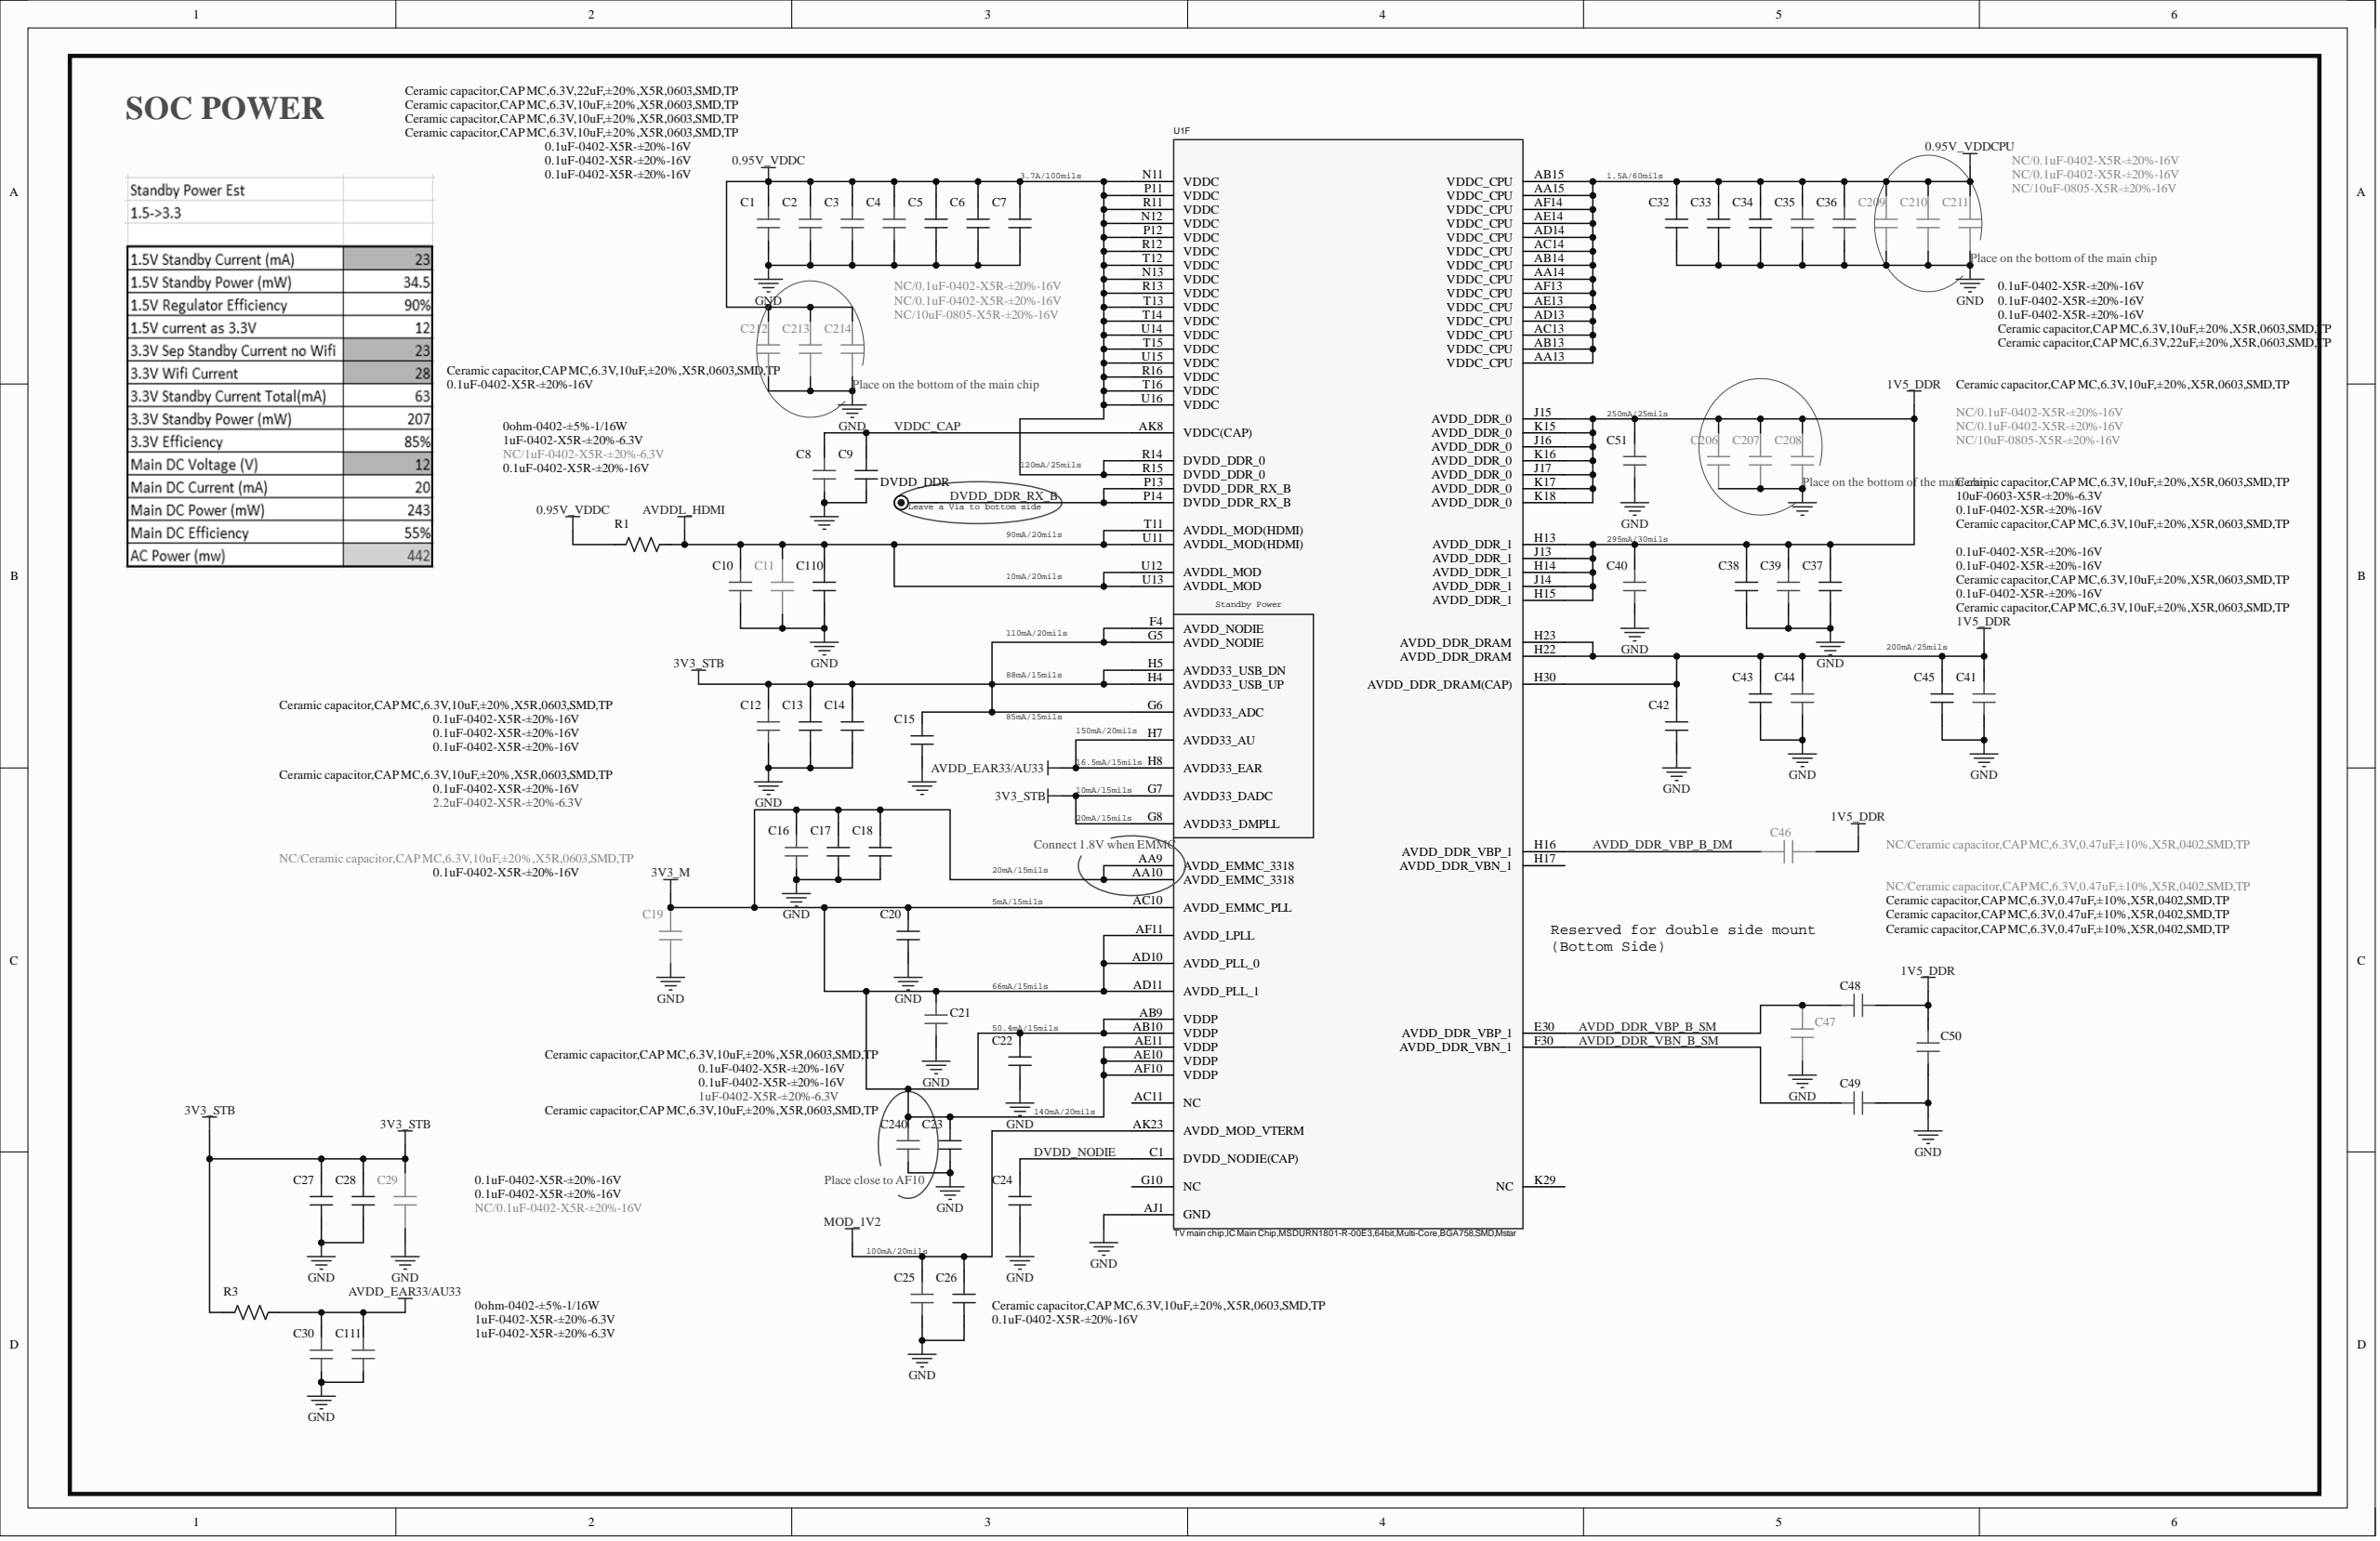Circuit board | Altium Designer | 1029 parts | 642 nets | one sheet of the schematic
Parts on this sheet (reference | value | footprint):
C1 | Ceramic capacitor,CAP MC,6.3V,22uF,±20%,X5R,0603,SMD,TP | C0603
C2 | Ceramic capacitor,CAP MC,6.3V,10uF,±20%,X5R,0603,SMD,TP | C0603
C3 | Ceramic capacitor,CAP MC,6.3V,10uF,±20%,X5R,0603,SMD,TP | C0603
C4 | Ceramic capacitor,CAP MC,6.3V,10uF,±20%,X5R,0603,SMD,TP | C0603
C5 | 0.1uF-0402-X5R-±20%-16V | C0402
C6 | 0.1uF-0402-X5R-±20%-16V | C0402
C7 | 0.1uF-0402-X5R-±20%-16V | C0402
C8 | Ceramic capacitor,CAP MC,6.3V,10uF,±20%,X5R,0603,SMD,TP | C0603
C9 | 0.1uF-0402-X5R-±20%-16V | C0402
C10 | 1uF-0402-X5R-±20%-6.3V | C0402
C11 | NC/1uF-0402-X5R-±20%-6.3V | C0402
C12 | Ceramic capacitor,CAP MC,6.3V,10uF,±20%,X5R,0603,SMD,TP | C0603
C13 | 0.1uF-0402-X5R-±20%-16V | C0402
C14 | 0.1uF-0402-X5R-±20%-16V | C0402
C15 | 0.1uF-0402-X5R-±20%-16V | C0402
C16 | Ceramic capacitor,CAP MC,6.3V,10uF,±20%,X5R,0603,SMD,TP | C0603
C17 | 0.1uF-0402-X5R-±20%-16V | C0402
C18 | 2.2uF-0402-X5R-±20%-6.3V | C0402
C19 | NC/Ceramic capacitor,CAP MC,6.3V,10uF,±20%,X5R,0603,SMD,TP | C0603
C20 | 0.1uF-0402-X5R-±20%-16V | C0402
C21 | Ceramic capacitor,CAP MC,6.3V,10uF,±20%,X5R,0603,SMD,TP | C0603
C22 | 0.1uF-0402-X5R-±20%-16V | C0402
C23 | 0.1uF-0402-X5R-±20%-16V | C0402
C24 | 1uF-0402-X5R-±20%-6.3V | C0402
C25 | Ceramic capacitor,CAP MC,6.3V,10uF,±20%,X5R,0603,SMD,TP | C0603
C26 | 0.1uF-0402-X5R-±20%-16V | C0402
C27 | 0.1uF-0402-X5R-±20%-16V | C0402
C28 | 0.1uF-0402-X5R-±20%-16V | C0402
C29 | NC/0.1uF-0402-X5R-±20%-16V | C0402
C30 | 1uF-0402-X5R-±20%-6.3V | C0402
C32 | 0.1uF-0402-X5R-±20%-16V | C0402
C33 | 0.1uF-0402-X5R-±20%-16V | C0402
C34 | 0.1uF-0402-X5R-±20%-16V | C0402
C35 | Ceramic capacitor,CAP MC,6.3V,10uF,±20%,X5R,0603,SMD,TP | C0603
C36 | Ceramic capacitor,CAP MC,6.3V,22uF,±20%,X5R,0603,SMD,TP | C0603
C37 | 10uF-0603-X5R-±20%-6.3V | C0603
C38 | 0.1uF-0402-X5R-±20%-16V | C0402
C39 | Ceramic capacitor,CAP MC,6.3V,10uF,±20%,X5R,0603,SMD,TP | C0603
C40 | Ceramic capacitor,CAP MC,6.3V,10uF,±20%,X5R,0603,SMD,TP | C0603
C41 | Ceramic capacitor,CAP MC,6.3V,10uF,±20%,X5R,0603,SMD,TP | C0603
C42 | 0.1uF-0402-X5R-±20%-16V | C0402
C43 | 0.1uF-0402-X5R-±20%-16V | C0402
C44 | Ceramic capacitor,CAP MC,6.3V,10uF,±20%,X5R,0603,SMD,TP | C0603
C45 | 0.1uF-0402-X5R-±20%-16V | C0402
C46 | NC/Ceramic capacitor,CAP MC,6.3V,0.47uF,±10%,X5R,0402,SMD,TP | C0402
C47 | NC/Ceramic capacitor,CAP MC,6.3V,0.47uF,±10%,X5R,0402,SMD,TP | C0402
C48 | Ceramic capacitor,CAP MC,6.3V,0.47uF,±10%,X5R,0402,SMD,TP | C0402
C49 | Ceramic capacitor,CAP MC,6.3V,0.47uF,±10%,X5R,0402,SMD,TP | C0402
C50 | Ceramic capacitor,CAP MC,6.3V,0.47uF,±10%,X5R,0402,SMD,TP | C0402
C51 | Ceramic capacitor,CAP MC,6.3V,10uF,±20%,X5R,0603,SMD,TP | C0603
C110 | 0.1uF-0402-X5R-±20%-16V | C0402
C111 | 1uF-0402-X5R-±20%-6.3V | C0402
C206 | NC/0.1uF-0402-X5R-±20%-16V | C0402
C207 | NC/0.1uF-0402-X5R-±20%-16V | C0402
C208 | NC/10uF-0805-X5R-±20%-16V | C0805
C209 | NC/0.1uF-0402-X5R-±20%-16V | C0402
C210 | NC/0.1uF-0402-X5R-±20%-16V | C0402
C211 | NC/10uF-0805-X5R-±20%-16V | C0805
C212 | NC/0.1uF-0402-X5R-±20%-16V | C0402
C213 | NC/0.1uF-0402-X5R-±20%-16V | C0402
C214 | NC/10uF-0805-X5R-±20%-16V | C0805
C240 | Ceramic capacitor,CAP MC,6.3V,10uF,±20%,X5R,0603,SMD,TP | C0603
DVDD_DDR | TEST | TP-20
R1 | 0ohm-0402-±5%-1/16W | R0402
R3 | 0ohm-0402-±5%-1/16W | R0402
U1 | TV main chip,IC Main Chip,MSDURN1801-R-00E3,64bit,Multi-Core,BGA758,SMD,Mstar | BGA758/0.65
Nets of these parts (net: part-pin ...):
VDDC_CAP: C8-2 C9-1 U1-AK8
MOD_1V2: C25-2 C26-1 U1-AK23
GND: C1-1 C2-1 C3-1 C4-1 C5-2 C6-2 C7-2 C8-1 C9-2 C10-1 C11-1 C12-1 C13-2 C14-2 C15-2 C16-1 C17-2 C18-2 C19-1 C20-2 C21-1 C22-2 C23-2 C24-2 C25-1 C26-2 C27-2 C28-2 C29-2 C30-1 C32-2 C33-2 C34-2 C35-1 C36-1 C37-2 C38-2 C39-1 C40-1 C41-1 C42-2 C43-2 C44-1 C45-2 C47-1 C49-1 C50-2 C51-1 C110-2 C111-1 C206-2 C207-2 C208-2 C209-2 C210-2 C211-2 C212-2 C213-2 C214-2 C240-1 U1-AJ1 U1-C3 U1-C9 U1-C10 U1-C16 U1-C19 U1-C24 U1-C26
DVDD_NODIE: C24-1 U1-C1
DVDD_DDR_RX_B: DVDD_DDR-1 U1-P13 U1-P14
AVDDL_HDMI: C10-2 C11-2 C110-1 R1-2 U1-T11 U1-U11 U1-U12 U1-U13
AVDD_EAR33/AU33: C30-2 C111-2 R3-2 U1-H7 U1-H8
AVDD_DDR_VBP_B_SM: C47-2 C48-2 U1-E30
AVDD_DDR_VBP_B_DM: C46-1 U1-H16
AVDD_DDR_VBN_B_SM: C49-2 U1-F30
3V3_STB: C12-2 C13-1 C14-1 C15-1 C27-1 C28-1 C29-1 R3-1 U1-F4 U1-G5 U1-G6 U1-G7 U1-G8 U1-H4 U1-H5
3V3_M: C16-2 C17-1 C18-1 C19-2 C20-1 C21-2 C22-1 C23-1 C240-2 U1-AA9 U1-AA10 U1-AB9 U1-AB10 U1-AC10 U1-AD10 U1-AD11 U1-AE10 U1-AE11 U1-AF10 U1-AF11
1V5_DDR: C37-1 C38-1 C39-2 C40-2 C41-2 C42-1 C43-1 C44-2 C45-1 C46-2 C48-1 C50-1 C51-2 C206-1 C207-1 C208-1 U1-H13 U1-H14 U1-H15 U1-H22 U1-H23 U1-H30 U1-J13 U1-J14 U1-J15 U1-J16 U1-J17 U1-K15 U1-K16 U1-K17 U1-K18
0.95V_VDDCPU: C32-1 C33-1 C34-1 C35-2 C36-2 C209-1 C210-1 C211-1 U1-AA13 U1-AA14 U1-AA15 U1-AB13 U1-AB14 U1-AB15 U1-AC13 U1-AC14 U1-AD13 U1-AD14 U1-AE13 U1-AE14 U1-AF13 U1-AF14
0.95V_VDDC: C1-2 C2-2 C3-2 C4-2 C5-1 C6-1 C7-1 C212-1 C213-1 C214-1 R1-1 U1-N11 U1-N12 U1-N13 U1-P11 U1-P12 U1-R11 U1-R12 U1-R13 U1-R14 U1-R15 U1-R16 U1-T12 U1-T13 U1-T14 U1-T15 U1-T16 U1-U14 U1-U15 U1-U16